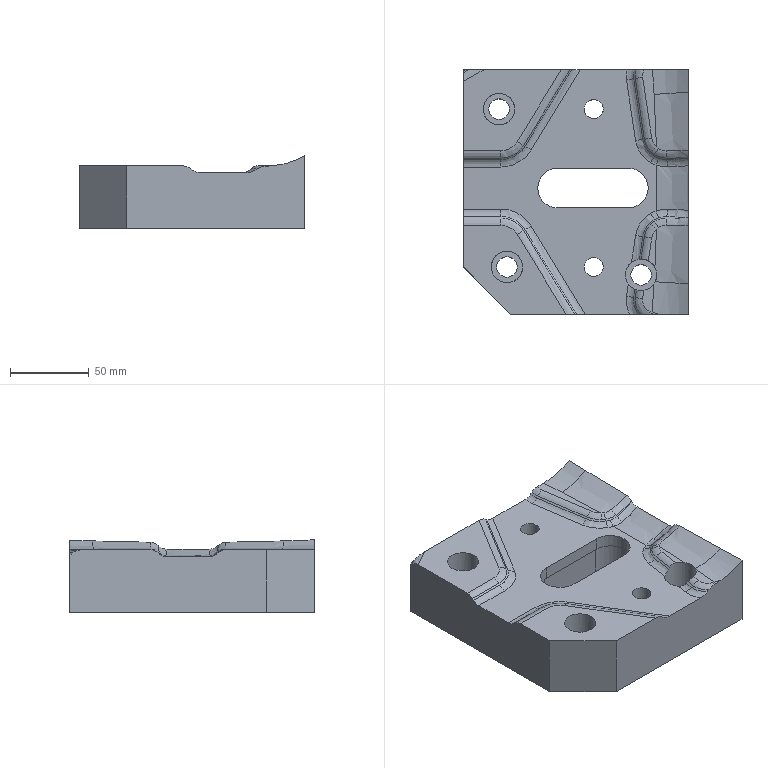Part | NX | features solid 2 | 1 solid | 98 faces | box 142.5 x 155.001 x 45.841 mm | volume 709213 mm3 | spline 77 | plane 13 | cylinder 8 | commonest cylinder face diameters 13 x3 20 x3 12 x2